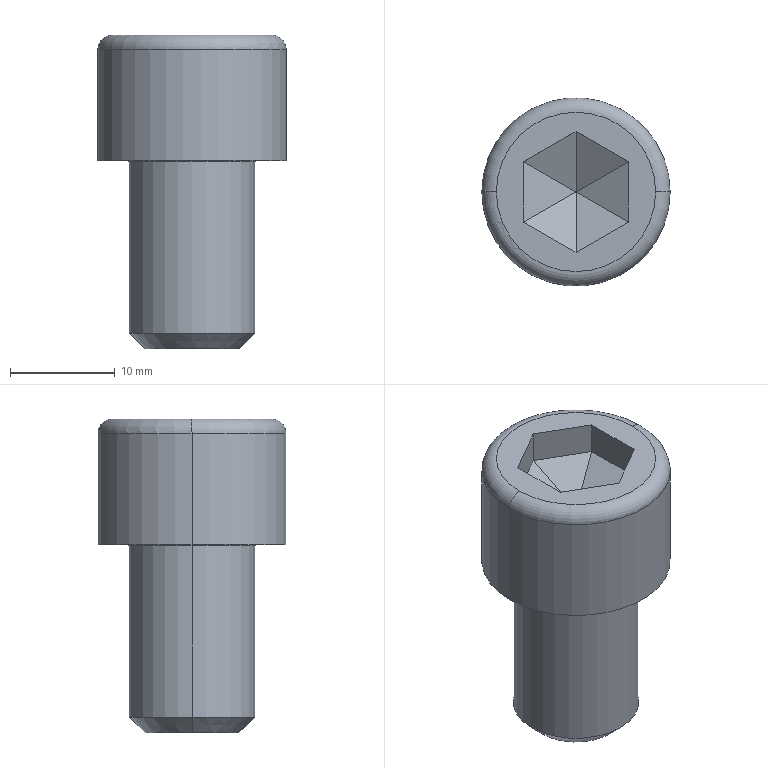Part | SolidWorks | features Chamfer 2, Fillet 2, ICE 2, Extrusion 1, RefAxis 1 | 1 solid | 26 faces | box 18 x 18 x 30 mm | volume 4675 mm3 | plane 16 | torus 4 | cylinder 4 | cone 2 | commonest cylinder face diameters 12 x2 18 x2
STEP:
#1=CARTESIAN_POINT('',(-6.1,0.,0.));
#2=VERTEX_POINT('',#1);
#3=CARTESIAN_POINT('',(6.1,0.,0.));
#4=VERTEX_POINT('',#3);
#5=CARTESIAN_POINT('',(0.,0.,0.));
#6=DIRECTION('',(0.,0.,1.));
#7=DIRECTION('',(1.,0.,0.));
#8=AXIS2_PLACEMENT_3D('',#5,#6,#7);
#9=CIRCLE('',#8,6.1);
#10=EDGE_CURVE('',#2,#4,#9,.T.);
#11=ORIENTED_EDGE('',*,*,#10,.F.);
#12=CARTESIAN_POINT('',(-6.,0.,-0.1));
#13=VERTEX_POINT('',#12);
#14=CARTESIAN_POINT('',(-6.1,0.,-0.1));
#15=DIRECTION('',(0.,1.,0.));
#16=DIRECTION('',(-1.,0.,0.));
#17=AXIS2_PLACEMENT_3D('',#14,#15,#16);
#18=CIRCLE('',#17,0.1);
#19=EDGE_CURVE('',#2,#13,#18,.T.);
#20=ORIENTED_EDGE('',*,*,#19,.T.);
#21=CARTESIAN_POINT('',(6.,0.,-0.1));
#22=VERTEX_POINT('',#21);
#23=CARTESIAN_POINT('',(0.,0.,-0.1));
#24=DIRECTION('',(0.,0.,-1.));
#25=DIRECTION('',(1.,0.,0.));
#26=AXIS2_PLACEMENT_3D('',#23,#24,#25);
#27=CIRCLE('',#26,6.);
#28=EDGE_CURVE('',#22,#13,#27,.T.);
#29=ORIENTED_EDGE('',*,*,#28,.F.);
#30=CARTESIAN_POINT('',(6.1,0.,-0.1));
#31=DIRECTION('',(0.,-1.,0.));
#32=DIRECTION('',(0.,0.,-1.));
#33=AXIS2_PLACEMENT_3D('',#30,#31,#32);
#34=CIRCLE('',#33,0.1);
#35=EDGE_CURVE('',#4,#22,#34,.T.);
#36=ORIENTED_EDGE('',*,*,#35,.F.);
#37=EDGE_LOOP('',(#11,#20,#29,#36));
#38=FACE_OUTER_BOUND('',#37,.T.);
#39=CARTESIAN_POINT('',(0.,0.,-0.1));
#40=DIRECTION('',(0.,0.,1.));
#41=DIRECTION('',(1.,0.,0.));
#42=AXIS2_PLACEMENT_3D('',#39,#40,#41);
#43=TOROIDAL_SURFACE('',#42,6.1,0.1);
#44=ADVANCED_FACE('',(#38),#43,.F.);
#45=CARTESIAN_POINT('',(-9.,0.,10.615));
#46=VERTEX_POINT('',#45);
#47=CARTESIAN_POINT('',(9.,0.,10.615));
#48=VERTEX_POINT('',#47);
#49=CARTESIAN_POINT('',(0.,0.,10.615));
#50=DIRECTION('',(0.,0.,-1.));
#51=DIRECTION('',(1.,0.,0.));
#52=AXIS2_PLACEMENT_3D('',#49,#50,#51);
#53=CIRCLE('',#52,9.);
#54=EDGE_CURVE('',#46,#48,#53,.T.);
#55=ORIENTED_EDGE('',*,*,#54,.F.);
#56=CARTESIAN_POINT('',(-7.615,0.,12.));
#57=VERTEX_POINT('',#56);
#58=CARTESIAN_POINT('',(-7.615,0.,10.615));
#59=DIRECTION('',(0.,1.,0.));
#60=DIRECTION('',(-1.,0.,0.));
#61=AXIS2_PLACEMENT_3D('',#58,#59,#60);
#62=CIRCLE('',#61,1.385);
#63=EDGE_CURVE('',#46,#57,#62,.T.);
#64=ORIENTED_EDGE('',*,*,#63,.T.);
#65=CARTESIAN_POINT('',(7.615,0.,12.));
#66=VERTEX_POINT('',#65);
#67=CARTESIAN_POINT('',(0.,0.,12.));
#68=DIRECTION('',(0.,0.,1.));
#69=DIRECTION('',(1.,0.,0.));
#70=AXIS2_PLACEMENT_3D('',#67,#68,#69);
#71=CIRCLE('',#70,7.615);
#72=EDGE_CURVE('',#66,#57,#71,.T.);
#73=ORIENTED_EDGE('',*,*,#72,.F.);
#74=CARTESIAN_POINT('',(7.615,0.,10.615));
#75=DIRECTION('',(0.,-1.,0.));
#76=DIRECTION('',(0.,0.,-1.));
#77=AXIS2_PLACEMENT_3D('',#74,#75,#76);
#78=CIRCLE('',#77,1.385);
#79=EDGE_CURVE('',#48,#66,#78,.T.);
#80=ORIENTED_EDGE('',*,*,#79,.F.);
#81=EDGE_LOOP('',(#55,#64,#73,#80));
#82=FACE_OUTER_BOUND('',#81,.T.);
#83=CARTESIAN_POINT('',(0.,0.,10.615));
#84=DIRECTION('',(0.,0.,1.));
#85=DIRECTION('',(1.,0.,0.));
#86=AXIS2_PLACEMENT_3D('',#83,#84,#85);
#87=TOROIDAL_SURFACE('',#86,7.615,1.385);
#88=ADVANCED_FACE('',(#82),#87,.T.);
#89=CARTESIAN_POINT('',(-4.5,0.,-18.));
#90=VERTEX_POINT('',#89);
#91=CARTESIAN_POINT('',(4.5,0.,-18.));
#92=VERTEX_POINT('',#91);
#93=CARTESIAN_POINT('',(0.,0.,-18.));
#94=DIRECTION('',(0.,0.,-1.));
#95=DIRECTION('',(-1.,0.,0.));
#96=AXIS2_PLACEMENT_3D('',#93,#94,#95);
#97=CIRCLE('',#96,4.5);
#98=EDGE_CURVE('',#90,#92,#97,.T.);
#99=ORIENTED_EDGE('',*,*,#98,.F.);
#100=CARTESIAN_POINT('',(-6.,0.,-16.5));
#101=VERTEX_POINT('',#100);
#102=CARTESIAN_POINT('',(-4.5,0.,-18.));
#103=DIRECTION('',(-0.7071,0.,0.7071));
#104=VECTOR('',#103,1000.);
#105=LINE('',#102,#104);
#106=EDGE_CURVE('',#90,#101,#105,.T.);
#107=ORIENTED_EDGE('',*,*,#106,.T.);
#108=CARTESIAN_POINT('',(6.,0.,-16.5));
#109=VERTEX_POINT('',#108);
#110=CARTESIAN_POINT('',(0.,0.,-16.5));
#111=DIRECTION('',(0.,0.,1.));
#112=DIRECTION('',(-1.,0.,0.));
#113=AXIS2_PLACEMENT_3D('',#110,#111,#112);
#114=CIRCLE('',#113,6.);
#115=EDGE_CURVE('',#109,#101,#114,.T.);
#116=ORIENTED_EDGE('',*,*,#115,.F.);
#117=CARTESIAN_POINT('',(4.5,0.,-18.));
#118=DIRECTION('',(0.7071,0.,0.7071));
#119=VECTOR('',#118,1000.);
#120=LINE('',#117,#119);
#121=EDGE_CURVE('',#92,#109,#120,.T.);
#122=ORIENTED_EDGE('',*,*,#121,.F.);
#123=EDGE_LOOP('',(#99,#107,#116,#122));
#124=FACE_OUTER_BOUND('',#123,.T.);
#125=CARTESIAN_POINT('',(0.,0.,-18.));
#126=DIRECTION('',(0.,0.,1.));
#127=DIRECTION('',(1.,0.,0.));
#128=AXIS2_PLACEMENT_3D('',#125,#126,#127);
#129=CONICAL_SURFACE('',#128,4.5,0.7854);
#130=ADVANCED_FACE('',(#124),#129,.T.);
#131=ORIENTED_EDGE('',*,*,#115,.T.);
#132=CARTESIAN_POINT('',(-6.,0.,-18.));
#133=DIRECTION('',(0.,0.,1.));
#134=VECTOR('',#133,1000.);
#135=LINE('',#132,#134);
#136=EDGE_CURVE('',#101,#13,#135,.T.);
#137=ORIENTED_EDGE('',*,*,#136,.T.);
#138=CARTESIAN_POINT('',(0.,0.,-0.1));
#139=DIRECTION('',(0.,0.,-1.));
#140=DIRECTION('',(1.,0.,0.));
#141=AXIS2_PLACEMENT_3D('',#138,#139,#140);
#142=CIRCLE('',#141,6.);
#143=EDGE_CURVE('',#13,#22,#142,.T.);
#144=ORIENTED_EDGE('',*,*,#143,.T.);
#145=CARTESIAN_POINT('',(6.,0.,-18.));
#146=DIRECTION('',(0.,0.,1.));
#147=VECTOR('',#146,1000.);
#148=LINE('',#145,#147);
#149=EDGE_CURVE('',#109,#22,#148,.T.);
#150=ORIENTED_EDGE('',*,*,#149,.F.);
#151=EDGE_LOOP('',(#131,#137,#144,#150));
#152=FACE_OUTER_BOUND('',#151,.T.);
#153=CARTESIAN_POINT('',(0.,0.,-18.));
#154=DIRECTION('',(0.,0.,1.));
#155=DIRECTION('',(1.,0.,0.));
#156=AXIS2_PLACEMENT_3D('',#153,#154,#155);
#157=CYLINDRICAL_SURFACE('',#156,6.);
#158=ADVANCED_FACE('',(#152),#157,.T.);
#159=ORIENTED_EDGE('',*,*,#54,.T.);
#160=CARTESIAN_POINT('',(9.,0.,0.));
#161=VERTEX_POINT('',#160);
#162=CARTESIAN_POINT('',(9.,0.,12.));
#163=DIRECTION('',(0.,0.,-1.));
#164=VECTOR('',#163,1000.);
#165=LINE('',#162,#164);
#166=EDGE_CURVE('',#48,#161,#165,.T.);
#167=ORIENTED_EDGE('',*,*,#166,.T.);
#168=CARTESIAN_POINT('',(-9.,0.,0.));
#169=VERTEX_POINT('',#168);
#170=CARTESIAN_POINT('',(0.,0.,0.));
#171=DIRECTION('',(0.,0.,1.));
#172=DIRECTION('',(1.,0.,0.));
#173=AXIS2_PLACEMENT_3D('',#170,#171,#172);
#174=CIRCLE('',#173,9.);
#175=EDGE_CURVE('',#161,#169,#174,.T.);
#176=ORIENTED_EDGE('',*,*,#175,.T.);
#177=CARTESIAN_POINT('',(-9.,0.,12.));
#178=DIRECTION('',(0.,0.,-1.));
#179=VECTOR('',#178,1000.);
#180=LINE('',#177,#179);
#181=EDGE_CURVE('',#46,#169,#180,.T.);
#182=ORIENTED_EDGE('',*,*,#181,.F.);
#183=EDGE_LOOP('',(#159,#167,#176,#182));
#184=FACE_OUTER_BOUND('',#183,.T.);
#185=CARTESIAN_POINT('',(0.,0.,12.));
#186=DIRECTION('',(0.,0.,-1.));
#187=DIRECTION('',(-1.,0.,0.));
#188=AXIS2_PLACEMENT_3D('',#185,#186,#187);
#189=CYLINDRICAL_SURFACE('',#188,9.);
#190=ADVANCED_FACE('',(#184),#189,.T.);
#191=CARTESIAN_POINT('',(0.,0.,0.));
#192=DIRECTION('',(0.,0.,1.));
#193=DIRECTION('',(1.,0.,0.));
#194=AXIS2_PLACEMENT_3D('',#191,#192,#193);
#195=CIRCLE('',#194,6.1);
#196=EDGE_CURVE('',#4,#2,#195,.T.);
#197=ORIENTED_EDGE('',*,*,#196,.T.);
#198=ORIENTED_EDGE('',*,*,#10,.T.);
#199=EDGE_LOOP('',(#197,#198));
#200=FACE_BOUND('',#199,.T.);
#201=CARTESIAN_POINT('',(0.,0.,0.));
#202=DIRECTION('',(0.,0.,1.));
#203=DIRECTION('',(1.,0.,0.));
#204=AXIS2_PLACEMENT_3D('',#201,#202,#203);
#205=CIRCLE('',#204,9.);
#206=EDGE_CURVE('',#169,#161,#205,.T.);
#207=ORIENTED_EDGE('',*,*,#206,.F.);
#208=ORIENTED_EDGE('',*,*,#175,.F.);
#209=EDGE_LOOP('',(#207,#208));
#210=FACE_OUTER_BOUND('',#209,.T.);
#211=CARTESIAN_POINT('',(0.,0.,0.));
#212=DIRECTION('',(0.,0.,1.));
#213=DIRECTION('',(1.,0.,0.));
#214=AXIS2_PLACEMENT_3D('',#211,#212,#213);
#215=PLANE('',#214);
#216=ADVANCED_FACE('',(#200,#210),#215,.F.);
#217=ORIENTED_EDGE('',*,*,#166,.F.);
#218=CARTESIAN_POINT('',(0.,0.,10.615));
#219=DIRECTION('',(0.,0.,-1.));
#220=DIRECTION('',(1.,0.,0.));
#221=AXIS2_PLACEMENT_3D('',#218,#219,#220);
#222=CIRCLE('',#221,9.);
#223=EDGE_CURVE('',#48,#46,#222,.T.);
#224=ORIENTED_EDGE('',*,*,#223,.T.);
#225=ORIENTED_EDGE('',*,*,#181,.T.);
#226=ORIENTED_EDGE('',*,*,#206,.T.);
#227=EDGE_LOOP('',(#217,#224,#225,#226));
#228=FACE_OUTER_BOUND('',#227,.T.);
#229=CARTESIAN_POINT('',(0.,0.,12.));
#230=DIRECTION('',(0.,0.,-1.));
#231=DIRECTION('',(-1.,0.,0.));
#232=AXIS2_PLACEMENT_3D('',#229,#230,#231);
#233=CYLINDRICAL_SURFACE('',#232,9.);
#234=ADVANCED_FACE('',(#228),#233,.T.);
#235=ORIENTED_EDGE('',*,*,#72,.T.);
#236=CARTESIAN_POINT('',(0.,0.,12.));
#237=DIRECTION('',(0.,0.,1.));
#238=DIRECTION('',(1.,0.,0.));
#239=AXIS2_PLACEMENT_3D('',#236,#237,#238);
#240=CIRCLE('',#239,7.615);
#241=EDGE_CURVE('',#57,#66,#240,.T.);
#242=ORIENTED_EDGE('',*,*,#241,.T.);
#243=EDGE_LOOP('',(#235,#242));
#244=FACE_OUTER_BOUND('',#243,.T.);
#245=CARTESIAN_POINT('',(5.,-2.887,12.));
#246=VERTEX_POINT('',#245);
#247=CARTESIAN_POINT('',(5.,2.887,12.));
#248=VERTEX_POINT('',#247);
#249=CARTESIAN_POINT('',(5.,-2.887,12.));
#250=DIRECTION('',(0.,1.,0.));
#251=VECTOR('',#250,1000.);
#252=LINE('',#249,#251);
#253=EDGE_CURVE('',#246,#248,#252,.T.);
#254=ORIENTED_EDGE('',*,*,#253,.F.);
#255=CARTESIAN_POINT('',(0.,-5.774,12.));
#256=VERTEX_POINT('',#255);
#257=CARTESIAN_POINT('',(0.,-5.774,12.));
#258=DIRECTION('',(0.866,0.5,0.));
#259=VECTOR('',#258,1000.);
#260=LINE('',#257,#259);
#261=EDGE_CURVE('',#256,#246,#260,.T.);
#262=ORIENTED_EDGE('',*,*,#261,.F.);
#263=CARTESIAN_POINT('',(-5.,-2.887,12.));
#264=VERTEX_POINT('',#263);
#265=CARTESIAN_POINT('',(-5.,-2.887,12.));
#266=DIRECTION('',(0.866,-0.5,0.));
#267=VECTOR('',#266,1000.);
#268=LINE('',#265,#267);
#269=EDGE_CURVE('',#264,#256,#268,.T.);
#270=ORIENTED_EDGE('',*,*,#269,.F.);
#271=CARTESIAN_POINT('',(-5.,2.887,12.));
#272=VERTEX_POINT('',#271);
#273=CARTESIAN_POINT('',(-5.,2.887,12.));
#274=DIRECTION('',(0.,-1.,0.));
#275=VECTOR('',#274,1000.);
#276=LINE('',#273,#275);
#277=EDGE_CURVE('',#272,#264,#276,.T.);
#278=ORIENTED_EDGE('',*,*,#277,.F.);
#279=CARTESIAN_POINT('',(0.,5.774,12.));
#280=VERTEX_POINT('',#279);
#281=CARTESIAN_POINT('',(0.,5.774,12.));
#282=DIRECTION('',(-0.866,-0.5,0.));
#283=VECTOR('',#282,1000.);
#284=LINE('',#281,#283);
#285=EDGE_CURVE('',#280,#272,#284,.T.);
#286=ORIENTED_EDGE('',*,*,#285,.F.);
#287=CARTESIAN_POINT('',(5.,2.887,12.));
#288=DIRECTION('',(-0.866,0.5,0.));
#289=VECTOR('',#288,1000.);
#290=LINE('',#287,#289);
#291=EDGE_CURVE('',#248,#280,#290,.T.);
#292=ORIENTED_EDGE('',*,*,#291,.F.);
#293=EDGE_LOOP('',(#254,#262,#270,#278,#286,#292));
#294=FACE_BOUND('',#293,.T.);
#295=CARTESIAN_POINT('',(0.,0.,12.));
#296=DIRECTION('',(0.,0.,1.));
#297=DIRECTION('',(1.,0.,0.));
#298=AXIS2_PLACEMENT_3D('',#295,#296,#297);
#299=PLANE('',#298);
#300=ADVANCED_FACE('',(#244,#294),#299,.T.);
#301=CARTESIAN_POINT('',(5.,2.887,8.882));
#302=VERTEX_POINT('',#301);
#303=CARTESIAN_POINT('',(5.,2.887,6.));
#304=DIRECTION('',(0.,0.,1.));
#305=VECTOR('',#304,1000.);
#306=LINE('',#303,#305);
#307=EDGE_CURVE('',#302,#248,#306,.T.);
#308=ORIENTED_EDGE('',*,*,#307,.F.);
#309=CARTESIAN_POINT('',(5.,-2.887,8.882));
#310=VERTEX_POINT('',#309);
#311=CARTESIAN_POINT('',(5.,-2.887,8.882));
#312=DIRECTION('',(0.,-1.,0.));
#313=VECTOR('',#312,1000.);
#314=LINE('',#311,#313);
#315=EDGE_CURVE('',#302,#310,#314,.T.);
#316=ORIENTED_EDGE('',*,*,#315,.T.);
#317=CARTESIAN_POINT('',(5.,-2.887,6.));
#318=DIRECTION('',(0.,0.,1.));
#319=VECTOR('',#318,1000.);
#320=LINE('',#317,#319);
#321=EDGE_CURVE('',#310,#246,#320,.T.);
#322=ORIENTED_EDGE('',*,*,#321,.T.);
#323=ORIENTED_EDGE('',*,*,#253,.T.);
#324=EDGE_LOOP('',(#308,#316,#322,#323));
#325=FACE_OUTER_BOUND('',#324,.T.);
#326=CARTESIAN_POINT('',(5.,-2.887,6.));
#327=DIRECTION('',(1.,0.,0.));
#328=DIRECTION('',(0.,0.,-1.));
#329=AXIS2_PLACEMENT_3D('',#326,#327,#328);
#330=PLANE('',#329);
#331=ADVANCED_FACE('',(#325),#330,.F.);
#332=ORIENTED_EDGE('',*,*,#321,.F.);
#333=CARTESIAN_POINT('',(0.,-5.774,8.882));
#334=VERTEX_POINT('',#333);
#335=CARTESIAN_POINT('',(0.,-5.774,8.882));
#336=DIRECTION('',(-0.866,-0.5,0.));
#337=VECTOR('',#336,1000.);
#338=LINE('',#335,#337);
#339=EDGE_CURVE('',#310,#334,#338,.T.);
#340=ORIENTED_EDGE('',*,*,#339,.T.);
#341=CARTESIAN_POINT('',(0.,-5.774,6.));
#342=DIRECTION('',(0.,0.,1.));
#343=VECTOR('',#342,1000.);
#344=LINE('',#341,#343);
#345=EDGE_CURVE('',#334,#256,#344,.T.);
#346=ORIENTED_EDGE('',*,*,#345,.T.);
#347=ORIENTED_EDGE('',*,*,#261,.T.);
#348=EDGE_LOOP('',(#332,#340,#346,#347));
#349=FACE_OUTER_BOUND('',#348,.T.);
#350=CARTESIAN_POINT('',(0.,-5.774,6.));
#351=DIRECTION('',(0.5,-0.866,0.));
#352=DIRECTION('',(0.866,0.5,0.));
#353=AXIS2_PLACEMENT_3D('',#350,#351,#352);
#354=PLANE('',#353);
#355=ADVANCED_FACE('',(#349),#354,.F.);
#356=ORIENTED_EDGE('',*,*,#345,.F.);
#357=CARTESIAN_POINT('',(-5.,-2.887,8.882));
#358=VERTEX_POINT('',#357);
#359=CARTESIAN_POINT('',(-5.,-2.887,8.882));
#360=DIRECTION('',(-0.866,0.5,0.));
#361=VECTOR('',#360,1000.);
#362=LINE('',#359,#361);
#363=EDGE_CURVE('',#334,#358,#362,.T.);
#364=ORIENTED_EDGE('',*,*,#363,.T.);
#365=CARTESIAN_POINT('',(-5.,-2.887,6.));
#366=DIRECTION('',(0.,0.,1.));
#367=VECTOR('',#366,1000.);
#368=LINE('',#365,#367);
#369=EDGE_CURVE('',#358,#264,#368,.T.);
#370=ORIENTED_EDGE('',*,*,#369,.T.);
#371=ORIENTED_EDGE('',*,*,#269,.T.);
#372=EDGE_LOOP('',(#356,#364,#370,#371));
#373=FACE_OUTER_BOUND('',#372,.T.);
#374=CARTESIAN_POINT('',(-5.,-2.887,6.));
#375=DIRECTION('',(-0.5,-0.866,0.));
#376=DIRECTION('',(0.866,-0.5,0.));
#377=AXIS2_PLACEMENT_3D('',#374,#375,#376);
#378=PLANE('',#377);
#379=ADVANCED_FACE('',(#373),#378,.F.);
#380=ORIENTED_EDGE('',*,*,#369,.F.);
#381=CARTESIAN_POINT('',(-5.,2.887,8.882));
#382=VERTEX_POINT('',#381);
#383=CARTESIAN_POINT('',(-5.,2.887,8.882));
#384=DIRECTION('',(0.,1.,0.));
#385=VECTOR('',#384,1000.);
#386=LINE('',#383,#385);
#387=EDGE_CURVE('',#358,#382,#386,.T.);
#388=ORIENTED_EDGE('',*,*,#387,.T.);
#389=CARTESIAN_POINT('',(-5.,2.887,6.));
#390=DIRECTION('',(0.,0.,1.));
#391=VECTOR('',#390,1000.);
#392=LINE('',#389,#391);
#393=EDGE_CURVE('',#382,#272,#392,.T.);
#394=ORIENTED_EDGE('',*,*,#393,.T.);
#395=ORIENTED_EDGE('',*,*,#277,.T.);
#396=EDGE_LOOP('',(#380,#388,#394,#395));
#397=FACE_OUTER_BOUND('',#396,.T.);
#398=CARTESIAN_POINT('',(-5.,2.887,6.));
#399=DIRECTION('',(-1.,0.,0.));
#400=DIRECTION('',(0.,0.,1.));
#401=AXIS2_PLACEMENT_3D('',#398,#399,#400);
#402=PLANE('',#401);
#403=ADVANCED_FACE('',(#397),#402,.F.);
#404=ORIENTED_EDGE('',*,*,#393,.F.);
#405=CARTESIAN_POINT('',(0.,5.774,8.882));
#406=VERTEX_POINT('',#405);
#407=CARTESIAN_POINT('',(0.,5.774,8.882));
#408=DIRECTION('',(0.866,0.5,0.));
#409=VECTOR('',#408,1000.);
#410=LINE('',#407,#409);
#411=EDGE_CURVE('',#382,#406,#410,.T.);
#412=ORIENTED_EDGE('',*,*,#411,.T.);
#413=CARTESIAN_POINT('',(0.,5.774,6.));
#414=DIRECTION('',(0.,0.,1.));
#415=VECTOR('',#414,1000.);
#416=LINE('',#413,#415);
#417=EDGE_CURVE('',#406,#280,#416,.T.);
#418=ORIENTED_EDGE('',*,*,#417,.T.);
#419=ORIENTED_EDGE('',*,*,#285,.T.);
#420=EDGE_LOOP('',(#404,#412,#418,#419));
#421=FACE_OUTER_BOUND('',#420,.T.);
#422=CARTESIAN_POINT('',(0.,5.774,6.));
#423=DIRECTION('',(-0.5,0.866,0.));
#424=DIRECTION('',(-0.866,-0.5,0.));
#425=AXIS2_PLACEMENT_3D('',#422,#423,#424);
#426=PLANE('',#425);
#427=ADVANCED_FACE('',(#421),#426,.F.);
#428=ORIENTED_EDGE('',*,*,#417,.F.);
#429=CARTESIAN_POINT('',(5.,2.887,8.882));
#430=DIRECTION('',(0.866,-0.5,0.));
#431=VECTOR('',#430,1000.);
#432=LINE('',#429,#431);
#433=EDGE_CURVE('',#406,#302,#432,.T.);
#434=ORIENTED_EDGE('',*,*,#433,.T.);
#435=ORIENTED_EDGE('',*,*,#307,.T.);
#436=ORIENTED_EDGE('',*,*,#291,.T.);
#437=EDGE_LOOP('',(#428,#434,#435,#436));
#438=FACE_OUTER_BOUND('',#437,.T.);
#439=CARTESIAN_POINT('',(5.,2.887,6.));
#440=DIRECTION('',(0.5,0.866,0.));
#441=DIRECTION('',(-0.866,0.5,0.));
#442=AXIS2_PLACEMENT_3D('',#439,#440,#441);
#443=PLANE('',#442);
#444=ADVANCED_FACE('',(#438),#443,.F.);
#445=CARTESIAN_POINT('',(0.,0.009814,6.));
#446=VERTEX_POINT('',#445);
#447=CARTESIAN_POINT('',(-0.008499,0.004907,6.));
#448=VERTEX_POINT('',#447);
#449=CARTESIAN_POINT('',(-0.00425,0.00736,6.));
#450=DIRECTION('',(-0.866,-0.5,0.));
#451=VECTOR('',#450,1000.);
#452=LINE('',#449,#451);
#453=EDGE_CURVE('',#446,#448,#452,.T.);
#454=ORIENTED_EDGE('',*,*,#453,.T.);
#455=CARTESIAN_POINT('',(-0.008499,-0.004907,6.));
#456=VERTEX_POINT('',#455);
#457=CARTESIAN_POINT('',(-0.008499,0.,6.));
#458=DIRECTION('',(0.,-1.,0.));
#459=VECTOR('',#458,1000.);
#460=LINE('',#457,#459);
#461=EDGE_CURVE('',#448,#456,#460,.T.);
#462=ORIENTED_EDGE('',*,*,#461,.T.);
#463=CARTESIAN_POINT('',(0.,-0.009814,6.));
#464=VERTEX_POINT('',#463);
#465=CARTESIAN_POINT('',(-0.00425,-0.00736,6.));
#466=DIRECTION('',(0.866,-0.5,0.));
#467=VECTOR('',#466,1000.);
#468=LINE('',#465,#467);
#469=EDGE_CURVE('',#456,#464,#468,.T.);
#470=ORIENTED_EDGE('',*,*,#469,.T.);
#471=CARTESIAN_POINT('',(0.008499,-0.004907,6.));
#472=VERTEX_POINT('',#471);
#473=CARTESIAN_POINT('',(0.00425,-0.00736,6.));
#474=DIRECTION('',(0.866,0.5,0.));
#475=VECTOR('',#474,1000.);
#476=LINE('',#473,#475);
#477=EDGE_CURVE('',#464,#472,#476,.T.);
#478=ORIENTED_EDGE('',*,*,#477,.T.);
#479=CARTESIAN_POINT('',(0.008499,0.004907,6.));
#480=VERTEX_POINT('',#479);
#481=CARTESIAN_POINT('',(0.008499,0.,6.));
#482=DIRECTION('',(0.,1.,0.));
#483=VECTOR('',#482,1000.);
#484=LINE('',#481,#483);
#485=EDGE_CURVE('',#472,#480,#484,.T.);
#486=ORIENTED_EDGE('',*,*,#485,.T.);
#487=CARTESIAN_POINT('',(0.00425,0.00736,6.));
#488=DIRECTION('',(-0.866,0.5,0.));
#489=VECTOR('',#488,1000.);
#490=LINE('',#487,#489);
#491=EDGE_CURVE('',#480,#446,#490,.T.);
#492=ORIENTED_EDGE('',*,*,#491,.T.);
#493=EDGE_LOOP('',(#454,#462,#470,#478,#486,#492));
#494=FACE_OUTER_BOUND('',#493,.T.);
#495=CARTESIAN_POINT('',(0.,0.,6.));
#496=DIRECTION('',(0.,0.,1.));
#497=DIRECTION('',(1.,0.,0.));
#498=AXIS2_PLACEMENT_3D('',#495,#496,#497);
#499=PLANE('',#498);
#500=ADVANCED_FACE('',(#494),#499,.T.);
#501=ORIENTED_EDGE('',*,*,#136,.F.);
#502=CARTESIAN_POINT('',(0.,0.,-16.5));
#503=DIRECTION('',(0.,0.,1.));
#504=DIRECTION('',(-1.,0.,0.));
#505=AXIS2_PLACEMENT_3D('',#502,#503,#504);
#506=CIRCLE('',#505,6.);
#507=EDGE_CURVE('',#101,#109,#506,.T.);
#508=ORIENTED_EDGE('',*,*,#507,.T.);
#509=ORIENTED_EDGE('',*,*,#149,.T.);
#510=ORIENTED_EDGE('',*,*,#28,.T.);
#511=EDGE_LOOP('',(#501,#508,#509,#510));
#512=FACE_OUTER_BOUND('',#511,.T.);
#513=CARTESIAN_POINT('',(0.,0.,-18.));
#514=DIRECTION('',(0.,0.,1.));
#515=DIRECTION('',(1.,0.,0.));
#516=AXIS2_PLACEMENT_3D('',#513,#514,#515);
#517=CYLINDRICAL_SURFACE('',#516,6.);
#518=ADVANCED_FACE('',(#512),#517,.T.);
#519=CARTESIAN_POINT('',(0.,0.,-18.));
#520=DIRECTION('',(0.,0.,-1.));
#521=DIRECTION('',(-1.,0.,0.));
#522=AXIS2_PLACEMENT_3D('',#519,#520,#521);
#523=CIRCLE('',#522,4.5);
#524=EDGE_CURVE('',#92,#90,#523,.T.);
#525=ORIENTED_EDGE('',*,*,#524,.T.);
#526=ORIENTED_EDGE('',*,*,#98,.T.);
#527=EDGE_LOOP('',(#525,#526));
#528=FACE_OUTER_BOUND('',#527,.T.);
#529=CARTESIAN_POINT('',(0.,0.,-18.));
#530=DIRECTION('',(0.,0.,-1.));
#531=DIRECTION('',(-1.,0.,0.));
#532=AXIS2_PLACEMENT_3D('',#529,#530,#531);
#533=PLANE('',#532);
#534=ADVANCED_FACE('',(#528),#533,.T.);
#535=ORIENTED_EDGE('',*,*,#106,.F.);
#536=ORIENTED_EDGE('',*,*,#524,.F.);
#537=ORIENTED_EDGE('',*,*,#121,.T.);
#538=ORIENTED_EDGE('',*,*,#507,.F.);
#539=EDGE_LOOP('',(#535,#536,#537,#538));
#540=FACE_OUTER_BOUND('',#539,.T.);
#541=CARTESIAN_POINT('',(0.,0.,-18.));
#542=DIRECTION('',(0.,0.,1.));
#543=DIRECTION('',(1.,0.,0.));
#544=AXIS2_PLACEMENT_3D('',#541,#542,#543);
#545=CONICAL_SURFACE('',#544,4.5,0.7854);
#546=ADVANCED_FACE('',(#540),#545,.T.);
#547=ORIENTED_EDGE('',*,*,#63,.F.);
#548=ORIENTED_EDGE('',*,*,#223,.F.);
#549=ORIENTED_EDGE('',*,*,#79,.T.);
#550=ORIENTED_EDGE('',*,*,#241,.F.);
#551=EDGE_LOOP('',(#547,#548,#549,#550));
#552=FACE_OUTER_BOUND('',#551,.T.);
#553=CARTESIAN_POINT('',(0.,0.,10.615));
#554=DIRECTION('',(0.,0.,1.));
#555=DIRECTION('',(1.,0.,0.));
#556=AXIS2_PLACEMENT_3D('',#553,#554,#555);
#557=TOROIDAL_SURFACE('',#556,7.615,1.385);
#558=ADVANCED_FACE('',(#552),#557,.T.);
#559=CARTESIAN_POINT('',(0.006799,-0.003926,5.999));
#560=DIRECTION('',(-0.7746,0.4472,-0.4472));
#561=VECTOR('',#560,1000.);
#562=LINE('',#559,#561);
#563=EDGE_CURVE('',#310,#472,#562,.T.);
#564=ORIENTED_EDGE('',*,*,#563,.F.);
#565=ORIENTED_EDGE('',*,*,#315,.F.);
#566=CARTESIAN_POINT('',(0.006799,0.003926,5.999));
#567=DIRECTION('',(0.7746,0.4472,0.4472));
#568=VECTOR('',#567,1000.);
#569=LINE('',#566,#568);
#570=EDGE_CURVE('',#480,#302,#569,.T.);
#571=ORIENTED_EDGE('',*,*,#570,.F.);
#572=ORIENTED_EDGE('',*,*,#485,.F.);
#573=EDGE_LOOP('',(#564,#565,#571,#572));
#574=FACE_OUTER_BOUND('',#573,.T.);
#575=CARTESIAN_POINT('',(0.008499,0.,6.));
#576=DIRECTION('',(0.5,0.,-0.866));
#577=DIRECTION('',(0.,1.,0.));
#578=AXIS2_PLACEMENT_3D('',#575,#576,#577);
#579=PLANE('',#578);
#580=ADVANCED_FACE('',(#574),#579,.F.);
#581=ORIENTED_EDGE('',*,*,#570,.T.);
#582=ORIENTED_EDGE('',*,*,#433,.F.);
#583=CARTESIAN_POINT('',(0.,0.007851,5.999));
#584=DIRECTION('',(0.,0.8944,0.4472));
#585=VECTOR('',#584,1000.);
#586=LINE('',#583,#585);
#587=EDGE_CURVE('',#446,#406,#586,.T.);
#588=ORIENTED_EDGE('',*,*,#587,.F.);
#589=ORIENTED_EDGE('',*,*,#491,.F.);
#590=EDGE_LOOP('',(#581,#582,#588,#589));
#591=FACE_OUTER_BOUND('',#590,.T.);
#592=CARTESIAN_POINT('',(0.00425,0.00736,6.));
#593=DIRECTION('',(0.25,0.433,-0.866));
#594=DIRECTION('',(-0.866,0.5,0.));
#595=AXIS2_PLACEMENT_3D('',#592,#593,#594);
#596=PLANE('',#595);
#597=ADVANCED_FACE('',(#591),#596,.F.);
#598=ORIENTED_EDGE('',*,*,#563,.T.);
#599=ORIENTED_EDGE('',*,*,#477,.F.);
#600=CARTESIAN_POINT('',(0.,-0.007851,5.999));
#601=DIRECTION('',(0.,0.8944,-0.4472));
#602=VECTOR('',#601,1000.);
#603=LINE('',#600,#602);
#604=EDGE_CURVE('',#334,#464,#603,.T.);
#605=ORIENTED_EDGE('',*,*,#604,.F.);
#606=ORIENTED_EDGE('',*,*,#339,.F.);
#607=EDGE_LOOP('',(#598,#599,#605,#606));
#608=FACE_OUTER_BOUND('',#607,.T.);
#609=CARTESIAN_POINT('',(0.00425,-0.00736,6.));
#610=DIRECTION('',(0.25,-0.433,-0.866));
#611=DIRECTION('',(0.866,0.5,0.));
#612=AXIS2_PLACEMENT_3D('',#609,#610,#611);
#613=PLANE('',#612);
#614=ADVANCED_FACE('',(#608),#613,.F.);
#615=ORIENTED_EDGE('',*,*,#587,.T.);
#616=ORIENTED_EDGE('',*,*,#411,.F.);
#617=CARTESIAN_POINT('',(-0.006799,0.003926,5.999));
#618=DIRECTION('',(-0.7746,0.4472,0.4472));
#619=VECTOR('',#618,1000.);
#620=LINE('',#617,#619);
#621=EDGE_CURVE('',#448,#382,#620,.T.);
#622=ORIENTED_EDGE('',*,*,#621,.F.);
#623=ORIENTED_EDGE('',*,*,#453,.F.);
#624=EDGE_LOOP('',(#615,#616,#622,#623));
#625=FACE_OUTER_BOUND('',#624,.T.);
#626=CARTESIAN_POINT('',(-0.00425,0.00736,6.));
#627=DIRECTION('',(-0.25,0.433,-0.866));
#628=DIRECTION('',(-0.866,-0.5,0.));
#629=AXIS2_PLACEMENT_3D('',#626,#627,#628);
#630=PLANE('',#629);
#631=ADVANCED_FACE('',(#625),#630,.F.);
#632=ORIENTED_EDGE('',*,*,#604,.T.);
#633=ORIENTED_EDGE('',*,*,#469,.F.);
#634=CARTESIAN_POINT('',(-0.006799,-0.003926,5.999));
#635=DIRECTION('',(0.7746,0.4472,-0.4472));
#636=VECTOR('',#635,1000.);
#637=LINE('',#634,#636);
#638=EDGE_CURVE('',#358,#456,#637,.T.);
#639=ORIENTED_EDGE('',*,*,#638,.F.);
#640=ORIENTED_EDGE('',*,*,#363,.F.);
#641=EDGE_LOOP('',(#632,#633,#639,#640));
#642=FACE_OUTER_BOUND('',#641,.T.);
#643=CARTESIAN_POINT('',(-0.00425,-0.00736,6.));
#644=DIRECTION('',(-0.25,-0.433,-0.866));
#645=DIRECTION('',(0.866,-0.5,0.));
#646=AXIS2_PLACEMENT_3D('',#643,#644,#645);
#647=PLANE('',#646);
#648=ADVANCED_FACE('',(#642),#647,.F.);
#649=ORIENTED_EDGE('',*,*,#621,.T.);
#650=ORIENTED_EDGE('',*,*,#387,.F.);
#651=ORIENTED_EDGE('',*,*,#638,.T.);
#652=ORIENTED_EDGE('',*,*,#461,.F.);
#653=EDGE_LOOP('',(#649,#650,#651,#652));
#654=FACE_OUTER_BOUND('',#653,.T.);
#655=CARTESIAN_POINT('',(-0.008499,0.,6.));
#656=DIRECTION('',(-0.5,0.,-0.866));
#657=DIRECTION('',(0.,-1.,0.));
#658=AXIS2_PLACEMENT_3D('',#655,#656,#657);
#659=PLANE('',#658);
#660=ADVANCED_FACE('',(#654),#659,.F.);
#661=ORIENTED_EDGE('',*,*,#19,.F.);
#662=ORIENTED_EDGE('',*,*,#196,.F.);
#663=ORIENTED_EDGE('',*,*,#35,.T.);
#664=ORIENTED_EDGE('',*,*,#143,.F.);
#665=EDGE_LOOP('',(#661,#662,#663,#664));
#666=FACE_OUTER_BOUND('',#665,.T.);
#667=CARTESIAN_POINT('',(0.,0.,-0.1));
#668=DIRECTION('',(0.,0.,1.));
#669=DIRECTION('',(1.,0.,0.));
#670=AXIS2_PLACEMENT_3D('',#667,#668,#669);
#671=TOROIDAL_SURFACE('',#670,6.1,0.1);
#672=ADVANCED_FACE('',(#666),#671,.F.);
#673=CLOSED_SHELL('',(#44,#88,#130,#158,#190,#216,#234,#300,#331,#355,#379,#403,#427,#444,#500,#518,#534,#546,#558,#580,#597,#614,#631,#648,#660,#672));
#674=MANIFOLD_SOLID_BREP('',#673);
#675=CARTESIAN_POINT('',(0.,0.,0.));
#676=DIRECTION('',(0.,0.,1.));
#677=DIRECTION('',(1.,0.,0.));
#678=AXIS2_PLACEMENT_3D('',#675,#676,#677);
#679=(LENGTH_UNIT()NAMED_UNIT(*)SI_UNIT(.MILLI.,.METRE.));
#680=UNCERTAINTY_MEASURE_WITH_UNIT(LENGTH_MEASURE(0.00001),#679,'','');
#681=(NAMED_UNIT(*)PLANE_ANGLE_UNIT()SI_UNIT($,.RADIAN.));
#682=(NAMED_UNIT(*)SI_UNIT($,.STERADIAN.)SOLID_ANGLE_UNIT());
#683=(GEOMETRIC_REPRESENTATION_CONTEXT(3)GLOBAL_UNCERTAINTY_ASSIGNED_CONTEXT((#680))GLOBAL_UNIT_ASSIGNED_CONTEXT((#679,#681,#682))REPRESENTATION_CONTEXT('',''));
#684=ADVANCED_BREP_SHAPE_REPRESENTATION('',(#674,#678),#683);